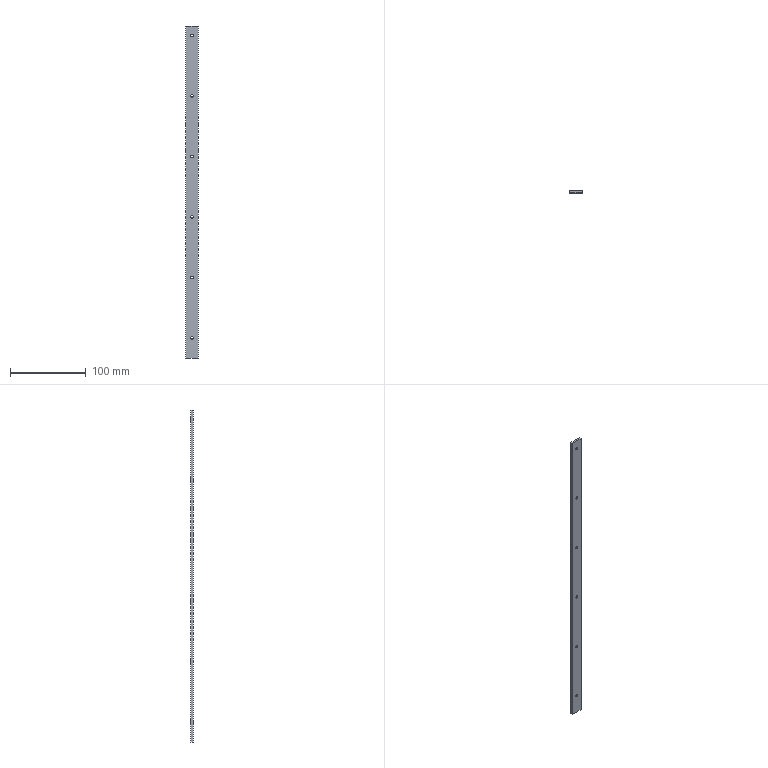Part | NX | features BREP 1 | 1 solid | 30 faces | box 16 x 3 x 439 mm | volume 20822 mm3 | cone 12 | cylinder 12 | plane 6 | commonest cylinder face diameters 3.4 x12
STEP:
#1=CARTESIAN_POINT('',(0.,1.5,203.85));
#2=VERTEX_POINT('',#1);
#3=CARTESIAN_POINT('',(0.,0.05,205.3));
#4=VERTEX_POINT('',#3);
#5=CARTESIAN_POINT('',(0.,1.5,203.85));
#6=DIRECTION('',(0.,0.7071,-0.7071));
#7=VECTOR('',#6,1000.);
#8=LINE('',#5,#7);
#9=EDGE_CURVE('',#2,#4,#8,.F.);
#10=ORIENTED_EDGE('',*,*,#9,.T.);
#11=CARTESIAN_POINT('',(0.,0.05,208.7));
#12=VERTEX_POINT('',#11);
#13=CARTESIAN_POINT('',(0.,0.05,207.));
#14=DIRECTION('',(0.,1.,0.));
#15=DIRECTION('',(0.,0.,1.));
#16=AXIS2_PLACEMENT_3D('',#13,#14,#15);
#17=CIRCLE('',#16,1.7);
#18=EDGE_CURVE('',#12,#4,#17,.T.);
#19=ORIENTED_EDGE('',*,*,#18,.F.);
#20=CARTESIAN_POINT('',(0.,1.5,210.15));
#21=VERTEX_POINT('',#20);
#22=CARTESIAN_POINT('',(0.,1.5,210.15));
#23=DIRECTION('',(0.,0.7071,0.7071));
#24=VECTOR('',#23,1000.);
#25=LINE('',#22,#24);
#26=EDGE_CURVE('',#21,#12,#25,.F.);
#27=ORIENTED_EDGE('',*,*,#26,.F.);
#28=CARTESIAN_POINT('',(0.,1.5,207.));
#29=DIRECTION('',(0.,1.,0.));
#30=DIRECTION('',(0.,0.,1.));
#31=AXIS2_PLACEMENT_3D('',#28,#29,#30);
#32=CIRCLE('',#31,3.15);
#33=EDGE_CURVE('',#21,#2,#32,.T.);
#34=ORIENTED_EDGE('',*,*,#33,.T.);
#35=EDGE_LOOP('',(#10,#19,#27,#34));
#36=FACE_BOUND('',#35,.T.);
#37=CARTESIAN_POINT('',(0.,1.5,207.));
#38=DIRECTION('',(0.,1.,0.));
#39=DIRECTION('',(0.,0.,1.));
#40=AXIS2_PLACEMENT_3D('',#37,#38,#39);
#41=CONICAL_SURFACE('',#40,3.15,0.7854);
#42=ADVANCED_FACE('',(#36),#41,.F.);
#43=CARTESIAN_POINT('',(0.,-1.5,205.3));
#44=VERTEX_POINT('',#43);
#45=CARTESIAN_POINT('',(0.,1.5,205.3));
#46=DIRECTION('',(0.,1.,0.));
#47=VECTOR('',#46,1000.);
#48=LINE('',#45,#47);
#49=EDGE_CURVE('',#4,#44,#48,.F.);
#50=ORIENTED_EDGE('',*,*,#49,.T.);
#51=CARTESIAN_POINT('',(0.,-1.5,208.7));
#52=VERTEX_POINT('',#51);
#53=CARTESIAN_POINT('',(0.,-1.5,207.));
#54=DIRECTION('',(0.,1.,0.));
#55=DIRECTION('',(0.,0.,1.));
#56=AXIS2_PLACEMENT_3D('',#53,#54,#55);
#57=CIRCLE('',#56,1.7);
#58=EDGE_CURVE('',#52,#44,#57,.T.);
#59=ORIENTED_EDGE('',*,*,#58,.F.);
#60=CARTESIAN_POINT('',(0.,1.5,208.7));
#61=DIRECTION('',(0.,1.,0.));
#62=VECTOR('',#61,1000.);
#63=LINE('',#60,#62);
#64=EDGE_CURVE('',#12,#52,#63,.F.);
#65=ORIENTED_EDGE('',*,*,#64,.F.);
#66=ORIENTED_EDGE('',*,*,#18,.T.);
#67=EDGE_LOOP('',(#50,#59,#65,#66));
#68=FACE_BOUND('',#67,.T.);
#69=CARTESIAN_POINT('',(0.,1.5,207.));
#70=DIRECTION('',(0.,1.,0.));
#71=DIRECTION('',(0.,0.,1.));
#72=AXIS2_PLACEMENT_3D('',#69,#70,#71);
#73=CYLINDRICAL_SURFACE('',#72,1.7);
#74=ADVANCED_FACE('',(#68),#73,.F.);
#75=CARTESIAN_POINT('',(0.,1.5,123.85));
#76=VERTEX_POINT('',#75);
#77=CARTESIAN_POINT('',(0.,0.05,125.3));
#78=VERTEX_POINT('',#77);
#79=CARTESIAN_POINT('',(0.,1.5,123.85));
#80=DIRECTION('',(0.,0.7071,-0.7071));
#81=VECTOR('',#80,1000.);
#82=LINE('',#79,#81);
#83=EDGE_CURVE('',#76,#78,#82,.F.);
#84=ORIENTED_EDGE('',*,*,#83,.T.);
#85=CARTESIAN_POINT('',(0.,0.05,128.7));
#86=VERTEX_POINT('',#85);
#87=CARTESIAN_POINT('',(0.,0.05,127.));
#88=DIRECTION('',(0.,1.,0.));
#89=DIRECTION('',(0.,0.,1.));
#90=AXIS2_PLACEMENT_3D('',#87,#88,#89);
#91=CIRCLE('',#90,1.7);
#92=EDGE_CURVE('',#86,#78,#91,.T.);
#93=ORIENTED_EDGE('',*,*,#92,.F.);
#94=CARTESIAN_POINT('',(0.,1.5,130.15));
#95=VERTEX_POINT('',#94);
#96=CARTESIAN_POINT('',(0.,1.5,130.15));
#97=DIRECTION('',(0.,0.7071,0.7071));
#98=VECTOR('',#97,1000.);
#99=LINE('',#96,#98);
#100=EDGE_CURVE('',#95,#86,#99,.F.);
#101=ORIENTED_EDGE('',*,*,#100,.F.);
#102=CARTESIAN_POINT('',(0.,1.5,127.));
#103=DIRECTION('',(0.,1.,0.));
#104=DIRECTION('',(0.,0.,1.));
#105=AXIS2_PLACEMENT_3D('',#102,#103,#104);
#106=CIRCLE('',#105,3.15);
#107=EDGE_CURVE('',#95,#76,#106,.T.);
#108=ORIENTED_EDGE('',*,*,#107,.T.);
#109=EDGE_LOOP('',(#84,#93,#101,#108));
#110=FACE_BOUND('',#109,.T.);
#111=CARTESIAN_POINT('',(0.,1.5,127.));
#112=DIRECTION('',(0.,1.,0.));
#113=DIRECTION('',(0.,0.,1.));
#114=AXIS2_PLACEMENT_3D('',#111,#112,#113);
#115=CONICAL_SURFACE('',#114,3.15,0.7854);
#116=ADVANCED_FACE('',(#110),#115,.F.);
#117=CARTESIAN_POINT('',(0.,-1.5,125.3));
#118=VERTEX_POINT('',#117);
#119=CARTESIAN_POINT('',(0.,1.5,125.3));
#120=DIRECTION('',(0.,1.,0.));
#121=VECTOR('',#120,1000.);
#122=LINE('',#119,#121);
#123=EDGE_CURVE('',#78,#118,#122,.F.);
#124=ORIENTED_EDGE('',*,*,#123,.T.);
#125=CARTESIAN_POINT('',(0.,-1.5,128.7));
#126=VERTEX_POINT('',#125);
#127=CARTESIAN_POINT('',(0.,-1.5,127.));
#128=DIRECTION('',(0.,1.,0.));
#129=DIRECTION('',(0.,0.,1.));
#130=AXIS2_PLACEMENT_3D('',#127,#128,#129);
#131=CIRCLE('',#130,1.7);
#132=EDGE_CURVE('',#126,#118,#131,.T.);
#133=ORIENTED_EDGE('',*,*,#132,.F.);
#134=CARTESIAN_POINT('',(0.,1.5,128.7));
#135=DIRECTION('',(0.,1.,0.));
#136=VECTOR('',#135,1000.);
#137=LINE('',#134,#136);
#138=EDGE_CURVE('',#86,#126,#137,.F.);
#139=ORIENTED_EDGE('',*,*,#138,.F.);
#140=ORIENTED_EDGE('',*,*,#92,.T.);
#141=EDGE_LOOP('',(#124,#133,#139,#140));
#142=FACE_BOUND('',#141,.T.);
#143=CARTESIAN_POINT('',(0.,1.5,127.));
#144=DIRECTION('',(0.,1.,0.));
#145=DIRECTION('',(0.,0.,1.));
#146=AXIS2_PLACEMENT_3D('',#143,#144,#145);
#147=CYLINDRICAL_SURFACE('',#146,1.7);
#148=ADVANCED_FACE('',(#142),#147,.F.);
#149=CARTESIAN_POINT('',(0.,1.5,43.85));
#150=VERTEX_POINT('',#149);
#151=CARTESIAN_POINT('',(0.,0.05,45.3));
#152=VERTEX_POINT('',#151);
#153=CARTESIAN_POINT('',(0.,1.5,43.85));
#154=DIRECTION('',(0.,0.7071,-0.7071));
#155=VECTOR('',#154,1000.);
#156=LINE('',#153,#155);
#157=EDGE_CURVE('',#150,#152,#156,.F.);
#158=ORIENTED_EDGE('',*,*,#157,.T.);
#159=CARTESIAN_POINT('',(0.,0.05,48.7));
#160=VERTEX_POINT('',#159);
#161=CARTESIAN_POINT('',(0.,0.05,47.));
#162=DIRECTION('',(0.,1.,0.));
#163=DIRECTION('',(0.,0.,1.));
#164=AXIS2_PLACEMENT_3D('',#161,#162,#163);
#165=CIRCLE('',#164,1.7);
#166=EDGE_CURVE('',#160,#152,#165,.T.);
#167=ORIENTED_EDGE('',*,*,#166,.F.);
#168=CARTESIAN_POINT('',(0.,1.5,50.15));
#169=VERTEX_POINT('',#168);
#170=CARTESIAN_POINT('',(0.,1.5,50.15));
#171=DIRECTION('',(0.,0.7071,0.7071));
#172=VECTOR('',#171,1000.);
#173=LINE('',#170,#172);
#174=EDGE_CURVE('',#169,#160,#173,.F.);
#175=ORIENTED_EDGE('',*,*,#174,.F.);
#176=CARTESIAN_POINT('',(0.,1.5,47.));
#177=DIRECTION('',(0.,1.,0.));
#178=DIRECTION('',(0.,0.,1.));
#179=AXIS2_PLACEMENT_3D('',#176,#177,#178);
#180=CIRCLE('',#179,3.15);
#181=EDGE_CURVE('',#169,#150,#180,.T.);
#182=ORIENTED_EDGE('',*,*,#181,.T.);
#183=EDGE_LOOP('',(#158,#167,#175,#182));
#184=FACE_BOUND('',#183,.T.);
#185=CARTESIAN_POINT('',(0.,1.5,47.));
#186=DIRECTION('',(0.,1.,0.));
#187=DIRECTION('',(0.,0.,1.));
#188=AXIS2_PLACEMENT_3D('',#185,#186,#187);
#189=CONICAL_SURFACE('',#188,3.15,0.7854);
#190=ADVANCED_FACE('',(#184),#189,.F.);
#191=CARTESIAN_POINT('',(0.,-1.5,45.3));
#192=VERTEX_POINT('',#191);
#193=CARTESIAN_POINT('',(0.,1.5,45.3));
#194=DIRECTION('',(0.,1.,0.));
#195=VECTOR('',#194,1000.);
#196=LINE('',#193,#195);
#197=EDGE_CURVE('',#152,#192,#196,.F.);
#198=ORIENTED_EDGE('',*,*,#197,.T.);
#199=CARTESIAN_POINT('',(0.,-1.5,48.7));
#200=VERTEX_POINT('',#199);
#201=CARTESIAN_POINT('',(0.,-1.5,47.));
#202=DIRECTION('',(0.,1.,0.));
#203=DIRECTION('',(0.,0.,1.));
#204=AXIS2_PLACEMENT_3D('',#201,#202,#203);
#205=CIRCLE('',#204,1.7);
#206=EDGE_CURVE('',#200,#192,#205,.T.);
#207=ORIENTED_EDGE('',*,*,#206,.F.);
#208=CARTESIAN_POINT('',(0.,1.5,48.7));
#209=DIRECTION('',(0.,1.,0.));
#210=VECTOR('',#209,1000.);
#211=LINE('',#208,#210);
#212=EDGE_CURVE('',#160,#200,#211,.F.);
#213=ORIENTED_EDGE('',*,*,#212,.F.);
#214=ORIENTED_EDGE('',*,*,#166,.T.);
#215=EDGE_LOOP('',(#198,#207,#213,#214));
#216=FACE_BOUND('',#215,.T.);
#217=CARTESIAN_POINT('',(0.,1.5,47.));
#218=DIRECTION('',(0.,1.,0.));
#219=DIRECTION('',(0.,0.,1.));
#220=AXIS2_PLACEMENT_3D('',#217,#218,#219);
#221=CYLINDRICAL_SURFACE('',#220,1.7);
#222=ADVANCED_FACE('',(#216),#221,.F.);
#223=CARTESIAN_POINT('',(0.,1.5,-36.15));
#224=VERTEX_POINT('',#223);
#225=CARTESIAN_POINT('',(0.,0.05,-34.7));
#226=VERTEX_POINT('',#225);
#227=CARTESIAN_POINT('',(0.,1.5,-36.15));
#228=DIRECTION('',(0.,0.7071,-0.7071));
#229=VECTOR('',#228,1000.);
#230=LINE('',#227,#229);
#231=EDGE_CURVE('',#224,#226,#230,.F.);
#232=ORIENTED_EDGE('',*,*,#231,.T.);
#233=CARTESIAN_POINT('',(0.,0.05,-31.3));
#234=VERTEX_POINT('',#233);
#235=CARTESIAN_POINT('',(0.,0.05,-33.));
#236=DIRECTION('',(0.,1.,0.));
#237=DIRECTION('',(0.,0.,1.));
#238=AXIS2_PLACEMENT_3D('',#235,#236,#237);
#239=CIRCLE('',#238,1.7);
#240=EDGE_CURVE('',#234,#226,#239,.T.);
#241=ORIENTED_EDGE('',*,*,#240,.F.);
#242=CARTESIAN_POINT('',(0.,1.5,-29.85));
#243=VERTEX_POINT('',#242);
#244=CARTESIAN_POINT('',(0.,1.5,-29.85));
#245=DIRECTION('',(0.,0.7071,0.7071));
#246=VECTOR('',#245,1000.);
#247=LINE('',#244,#246);
#248=EDGE_CURVE('',#243,#234,#247,.F.);
#249=ORIENTED_EDGE('',*,*,#248,.F.);
#250=CARTESIAN_POINT('',(0.,1.5,-33.));
#251=DIRECTION('',(0.,1.,0.));
#252=DIRECTION('',(0.,0.,1.));
#253=AXIS2_PLACEMENT_3D('',#250,#251,#252);
#254=CIRCLE('',#253,3.15);
#255=EDGE_CURVE('',#243,#224,#254,.T.);
#256=ORIENTED_EDGE('',*,*,#255,.T.);
#257=EDGE_LOOP('',(#232,#241,#249,#256));
#258=FACE_BOUND('',#257,.T.);
#259=CARTESIAN_POINT('',(0.,1.5,-33.));
#260=DIRECTION('',(0.,1.,0.));
#261=DIRECTION('',(0.,0.,1.));
#262=AXIS2_PLACEMENT_3D('',#259,#260,#261);
#263=CONICAL_SURFACE('',#262,3.15,0.7854);
#264=ADVANCED_FACE('',(#258),#263,.F.);
#265=CARTESIAN_POINT('',(0.,-1.5,-34.7));
#266=VERTEX_POINT('',#265);
#267=CARTESIAN_POINT('',(0.,1.5,-34.7));
#268=DIRECTION('',(0.,1.,0.));
#269=VECTOR('',#268,1000.);
#270=LINE('',#267,#269);
#271=EDGE_CURVE('',#226,#266,#270,.F.);
#272=ORIENTED_EDGE('',*,*,#271,.T.);
#273=CARTESIAN_POINT('',(0.,-1.5,-31.3));
#274=VERTEX_POINT('',#273);
#275=CARTESIAN_POINT('',(0.,-1.5,-33.));
#276=DIRECTION('',(0.,1.,0.));
#277=DIRECTION('',(0.,0.,1.));
#278=AXIS2_PLACEMENT_3D('',#275,#276,#277);
#279=CIRCLE('',#278,1.7);
#280=EDGE_CURVE('',#274,#266,#279,.T.);
#281=ORIENTED_EDGE('',*,*,#280,.F.);
#282=CARTESIAN_POINT('',(0.,1.5,-31.3));
#283=DIRECTION('',(0.,1.,0.));
#284=VECTOR('',#283,1000.);
#285=LINE('',#282,#284);
#286=EDGE_CURVE('',#234,#274,#285,.F.);
#287=ORIENTED_EDGE('',*,*,#286,.F.);
#288=ORIENTED_EDGE('',*,*,#240,.T.);
#289=EDGE_LOOP('',(#272,#281,#287,#288));
#290=FACE_BOUND('',#289,.T.);
#291=CARTESIAN_POINT('',(0.,1.5,-33.));
#292=DIRECTION('',(0.,1.,0.));
#293=DIRECTION('',(0.,0.,1.));
#294=AXIS2_PLACEMENT_3D('',#291,#292,#293);
#295=CYLINDRICAL_SURFACE('',#294,1.7);
#296=ADVANCED_FACE('',(#290),#295,.F.);
#297=CARTESIAN_POINT('',(0.,1.5,-116.15));
#298=VERTEX_POINT('',#297);
#299=CARTESIAN_POINT('',(0.,0.05,-114.7));
#300=VERTEX_POINT('',#299);
#301=CARTESIAN_POINT('',(0.,1.5,-116.15));
#302=DIRECTION('',(0.,0.7071,-0.7071));
#303=VECTOR('',#302,1000.);
#304=LINE('',#301,#303);
#305=EDGE_CURVE('',#298,#300,#304,.F.);
#306=ORIENTED_EDGE('',*,*,#305,.T.);
#307=CARTESIAN_POINT('',(0.,0.05,-111.3));
#308=VERTEX_POINT('',#307);
#309=CARTESIAN_POINT('',(0.,0.05,-113.));
#310=DIRECTION('',(0.,1.,0.));
#311=DIRECTION('',(0.,0.,1.));
#312=AXIS2_PLACEMENT_3D('',#309,#310,#311);
#313=CIRCLE('',#312,1.7);
#314=EDGE_CURVE('',#308,#300,#313,.T.);
#315=ORIENTED_EDGE('',*,*,#314,.F.);
#316=CARTESIAN_POINT('',(0.,1.5,-109.85));
#317=VERTEX_POINT('',#316);
#318=CARTESIAN_POINT('',(0.,1.5,-109.85));
#319=DIRECTION('',(0.,0.7071,0.7071));
#320=VECTOR('',#319,1000.);
#321=LINE('',#318,#320);
#322=EDGE_CURVE('',#317,#308,#321,.F.);
#323=ORIENTED_EDGE('',*,*,#322,.F.);
#324=CARTESIAN_POINT('',(0.,1.5,-113.));
#325=DIRECTION('',(0.,1.,0.));
#326=DIRECTION('',(0.,0.,1.));
#327=AXIS2_PLACEMENT_3D('',#324,#325,#326);
#328=CIRCLE('',#327,3.15);
#329=EDGE_CURVE('',#317,#298,#328,.T.);
#330=ORIENTED_EDGE('',*,*,#329,.T.);
#331=EDGE_LOOP('',(#306,#315,#323,#330));
#332=FACE_BOUND('',#331,.T.);
#333=CARTESIAN_POINT('',(0.,1.5,-113.));
#334=DIRECTION('',(0.,1.,0.));
#335=DIRECTION('',(0.,0.,1.));
#336=AXIS2_PLACEMENT_3D('',#333,#334,#335);
#337=CONICAL_SURFACE('',#336,3.15,0.7854);
#338=ADVANCED_FACE('',(#332),#337,.F.);
#339=CARTESIAN_POINT('',(0.,-1.5,-114.7));
#340=VERTEX_POINT('',#339);
#341=CARTESIAN_POINT('',(0.,1.5,-114.7));
#342=DIRECTION('',(0.,1.,0.));
#343=VECTOR('',#342,1000.);
#344=LINE('',#341,#343);
#345=EDGE_CURVE('',#300,#340,#344,.F.);
#346=ORIENTED_EDGE('',*,*,#345,.T.);
#347=CARTESIAN_POINT('',(0.,-1.5,-111.3));
#348=VERTEX_POINT('',#347);
#349=CARTESIAN_POINT('',(0.,-1.5,-113.));
#350=DIRECTION('',(0.,1.,0.));
#351=DIRECTION('',(0.,0.,1.));
#352=AXIS2_PLACEMENT_3D('',#349,#350,#351);
#353=CIRCLE('',#352,1.7);
#354=EDGE_CURVE('',#348,#340,#353,.T.);
#355=ORIENTED_EDGE('',*,*,#354,.F.);
#356=CARTESIAN_POINT('',(0.,1.5,-111.3));
#357=DIRECTION('',(0.,1.,0.));
#358=VECTOR('',#357,1000.);
#359=LINE('',#356,#358);
#360=EDGE_CURVE('',#308,#348,#359,.F.);
#361=ORIENTED_EDGE('',*,*,#360,.F.);
#362=ORIENTED_EDGE('',*,*,#314,.T.);
#363=EDGE_LOOP('',(#346,#355,#361,#362));
#364=FACE_BOUND('',#363,.T.);
#365=CARTESIAN_POINT('',(0.,1.5,-113.));
#366=DIRECTION('',(0.,1.,0.));
#367=DIRECTION('',(0.,0.,1.));
#368=AXIS2_PLACEMENT_3D('',#365,#366,#367);
#369=CYLINDRICAL_SURFACE('',#368,1.7);
#370=ADVANCED_FACE('',(#364),#369,.F.);
#371=CARTESIAN_POINT('',(0.,1.5,-196.15));
#372=VERTEX_POINT('',#371);
#373=CARTESIAN_POINT('',(0.,0.05,-194.7));
#374=VERTEX_POINT('',#373);
#375=CARTESIAN_POINT('',(0.,1.5,-196.15));
#376=DIRECTION('',(0.,0.7071,-0.7071));
#377=VECTOR('',#376,1000.);
#378=LINE('',#375,#377);
#379=EDGE_CURVE('',#372,#374,#378,.F.);
#380=ORIENTED_EDGE('',*,*,#379,.T.);
#381=CARTESIAN_POINT('',(0.,0.05,-191.3));
#382=VERTEX_POINT('',#381);
#383=CARTESIAN_POINT('',(0.,0.05,-193.));
#384=DIRECTION('',(0.,1.,0.));
#385=DIRECTION('',(0.,0.,1.));
#386=AXIS2_PLACEMENT_3D('',#383,#384,#385);
#387=CIRCLE('',#386,1.7);
#388=EDGE_CURVE('',#382,#374,#387,.T.);
#389=ORIENTED_EDGE('',*,*,#388,.F.);
#390=CARTESIAN_POINT('',(0.,1.5,-189.85));
#391=VERTEX_POINT('',#390);
#392=CARTESIAN_POINT('',(0.,1.5,-189.85));
#393=DIRECTION('',(0.,0.7071,0.7071));
#394=VECTOR('',#393,1000.);
#395=LINE('',#392,#394);
#396=EDGE_CURVE('',#391,#382,#395,.F.);
#397=ORIENTED_EDGE('',*,*,#396,.F.);
#398=CARTESIAN_POINT('',(0.,1.5,-193.));
#399=DIRECTION('',(0.,1.,0.));
#400=DIRECTION('',(0.,0.,1.));
#401=AXIS2_PLACEMENT_3D('',#398,#399,#400);
#402=CIRCLE('',#401,3.15);
#403=EDGE_CURVE('',#391,#372,#402,.T.);
#404=ORIENTED_EDGE('',*,*,#403,.T.);
#405=EDGE_LOOP('',(#380,#389,#397,#404));
#406=FACE_BOUND('',#405,.T.);
#407=CARTESIAN_POINT('',(0.,1.5,-193.));
#408=DIRECTION('',(0.,1.,0.));
#409=DIRECTION('',(0.,0.,1.));
#410=AXIS2_PLACEMENT_3D('',#407,#408,#409);
#411=CONICAL_SURFACE('',#410,3.15,0.7854);
#412=ADVANCED_FACE('',(#406),#411,.F.);
#413=CARTESIAN_POINT('',(0.,-1.5,-194.7));
#414=VERTEX_POINT('',#413);
#415=CARTESIAN_POINT('',(0.,1.5,-194.7));
#416=DIRECTION('',(0.,1.,0.));
#417=VECTOR('',#416,1000.);
#418=LINE('',#415,#417);
#419=EDGE_CURVE('',#374,#414,#418,.F.);
#420=ORIENTED_EDGE('',*,*,#419,.T.);
#421=CARTESIAN_POINT('',(0.,-1.5,-191.3));
#422=VERTEX_POINT('',#421);
#423=CARTESIAN_POINT('',(0.,-1.5,-193.));
#424=DIRECTION('',(0.,1.,0.));
#425=DIRECTION('',(0.,0.,1.));
#426=AXIS2_PLACEMENT_3D('',#423,#424,#425);
#427=CIRCLE('',#426,1.7);
#428=EDGE_CURVE('',#422,#414,#427,.T.);
#429=ORIENTED_EDGE('',*,*,#428,.F.);
#430=CARTESIAN_POINT('',(0.,1.5,-191.3));
#431=DIRECTION('',(0.,1.,0.));
#432=VECTOR('',#431,1000.);
#433=LINE('',#430,#432);
#434=EDGE_CURVE('',#382,#422,#433,.F.);
#435=ORIENTED_EDGE('',*,*,#434,.F.);
#436=ORIENTED_EDGE('',*,*,#388,.T.);
#437=EDGE_LOOP('',(#420,#429,#435,#436));
#438=FACE_BOUND('',#437,.T.);
#439=CARTESIAN_POINT('',(0.,1.5,-193.));
#440=DIRECTION('',(0.,1.,0.));
#441=DIRECTION('',(0.,0.,1.));
#442=AXIS2_PLACEMENT_3D('',#439,#440,#441);
#443=CYLINDRICAL_SURFACE('',#442,1.7);
#444=ADVANCED_FACE('',(#438),#443,.F.);
#445=CARTESIAN_POINT('',(8.,-1.5,-219.5));
#446=VERTEX_POINT('',#445);
#447=CARTESIAN_POINT('',(8.,1.5,-219.5));
#448=VERTEX_POINT('',#447);
#449=CARTESIAN_POINT('',(8.,-1.5,-219.5));
#450=DIRECTION('',(0.,1.,0.));
#451=VECTOR('',#450,1000.);
#452=LINE('',#449,#451);
#453=EDGE_CURVE('',#446,#448,#452,.T.);
#454=ORIENTED_EDGE('',*,*,#453,.F.);
#455=CARTESIAN_POINT('',(-8.,-1.5,-219.5));
#456=VERTEX_POINT('',#455);
#457=CARTESIAN_POINT('',(-8.,-1.5,-219.5));
#458=DIRECTION('',(1.,0.,0.));
#459=VECTOR('',#458,1000.);
#460=LINE('',#457,#459);
#461=EDGE_CURVE('',#456,#446,#460,.T.);
#462=ORIENTED_EDGE('',*,*,#461,.F.);
#463=CARTESIAN_POINT('',(-8.,1.5,-219.5));
#464=VERTEX_POINT('',#463);
#465=CARTESIAN_POINT('',(-8.,-1.5,-219.5));
#466=DIRECTION('',(0.,-1.,0.));
#467=VECTOR('',#466,1000.);
#468=LINE('',#465,#467);
#469=EDGE_CURVE('',#464,#456,#468,.T.);
#470=ORIENTED_EDGE('',*,*,#469,.F.);
#471=CARTESIAN_POINT('',(-8.,1.5,-219.5));
#472=DIRECTION('',(-1.,0.,0.));
#473=VECTOR('',#472,1000.);
#474=LINE('',#471,#473);
#475=EDGE_CURVE('',#448,#464,#474,.T.);
#476=ORIENTED_EDGE('',*,*,#475,.F.);
#477=EDGE_LOOP('',(#454,#462,#470,#476));
#478=FACE_BOUND('',#477,.T.);
#479=CARTESIAN_POINT('',(0.,0.,-219.5));
#480=DIRECTION('',(0.,0.,-1.));
#481=DIRECTION('',(-1.,0.,0.));
#482=AXIS2_PLACEMENT_3D('',#479,#480,#481);
#483=PLANE('',#482);
#484=ADVANCED_FACE('',(#478),#483,.T.);
#485=CARTESIAN_POINT('',(8.,-1.5,219.5));
#486=VERTEX_POINT('',#485);
#487=CARTESIAN_POINT('',(8.,1.5,219.5));
#488=VERTEX_POINT('',#487);
#489=CARTESIAN_POINT('',(8.,-1.5,219.5));
#490=DIRECTION('',(0.,1.,0.));
#491=VECTOR('',#490,1000.);
#492=LINE('',#489,#491);
#493=EDGE_CURVE('',#486,#488,#492,.T.);
#494=ORIENTED_EDGE('',*,*,#493,.T.);
#495=CARTESIAN_POINT('',(-8.,1.5,219.5));
#496=VERTEX_POINT('',#495);
#497=CARTESIAN_POINT('',(-8.,1.5,219.5));
#498=DIRECTION('',(-1.,0.,0.));
#499=VECTOR('',#498,1000.);
#500=LINE('',#497,#499);
#501=EDGE_CURVE('',#488,#496,#500,.T.);
#502=ORIENTED_EDGE('',*,*,#501,.T.);
#503=CARTESIAN_POINT('',(-8.,-1.5,219.5));
#504=VERTEX_POINT('',#503);
#505=CARTESIAN_POINT('',(-8.,-1.5,219.5));
#506=DIRECTION('',(0.,-1.,0.));
#507=VECTOR('',#506,1000.);
#508=LINE('',#505,#507);
#509=EDGE_CURVE('',#496,#504,#508,.T.);
#510=ORIENTED_EDGE('',*,*,#509,.T.);
#511=CARTESIAN_POINT('',(-8.,-1.5,219.5));
#512=DIRECTION('',(1.,0.,0.));
#513=VECTOR('',#512,1000.);
#514=LINE('',#511,#513);
#515=EDGE_CURVE('',#504,#486,#514,.T.);
#516=ORIENTED_EDGE('',*,*,#515,.T.);
#517=EDGE_LOOP('',(#494,#502,#510,#516));
#518=FACE_BOUND('',#517,.T.);
#519=CARTESIAN_POINT('',(0.,0.,219.5));
#520=DIRECTION('',(0.,0.,-1.));
#521=DIRECTION('',(-1.,0.,0.));
#522=AXIS2_PLACEMENT_3D('',#519,#520,#521);
#523=PLANE('',#522);
#524=ADVANCED_FACE('',(#518),#523,.F.);
#525=ORIENTED_EDGE('',*,*,#461,.T.);
#526=CARTESIAN_POINT('',(8.,-1.5,219.5));
#527=DIRECTION('',(0.,0.,-1.));
#528=VECTOR('',#527,1000.);
#529=LINE('',#526,#528);
#530=EDGE_CURVE('',#486,#446,#529,.T.);
#531=ORIENTED_EDGE('',*,*,#530,.F.);
#532=ORIENTED_EDGE('',*,*,#515,.F.);
#533=CARTESIAN_POINT('',(-8.,-1.5,219.5));
#534=DIRECTION('',(0.,0.,-1.));
#535=VECTOR('',#534,1000.);
#536=LINE('',#533,#535);
#537=EDGE_CURVE('',#504,#456,#536,.T.);
#538=ORIENTED_EDGE('',*,*,#537,.T.);
#539=EDGE_LOOP('',(#525,#531,#532,#538));
#540=FACE_BOUND('',#539,.T.);
#541=ORIENTED_EDGE('',*,*,#428,.T.);
#542=CARTESIAN_POINT('',(0.,-1.5,-193.));
#543=DIRECTION('',(0.,1.,0.));
#544=DIRECTION('',(0.,0.,1.));
#545=AXIS2_PLACEMENT_3D('',#542,#543,#544);
#546=CIRCLE('',#545,1.7);
#547=EDGE_CURVE('',#414,#422,#546,.T.);
#548=ORIENTED_EDGE('',*,*,#547,.T.);
#549=EDGE_LOOP('',(#541,#548));
#550=FACE_BOUND('',#549,.T.);
#551=ORIENTED_EDGE('',*,*,#354,.T.);
#552=CARTESIAN_POINT('',(0.,-1.5,-113.));
#553=DIRECTION('',(0.,1.,0.));
#554=DIRECTION('',(0.,0.,1.));
#555=AXIS2_PLACEMENT_3D('',#552,#553,#554);
#556=CIRCLE('',#555,1.7);
#557=EDGE_CURVE('',#340,#348,#556,.T.);
#558=ORIENTED_EDGE('',*,*,#557,.T.);
#559=EDGE_LOOP('',(#551,#558));
#560=FACE_BOUND('',#559,.T.);
#561=ORIENTED_EDGE('',*,*,#280,.T.);
#562=CARTESIAN_POINT('',(0.,-1.5,-33.));
#563=DIRECTION('',(0.,1.,0.));
#564=DIRECTION('',(0.,0.,1.));
#565=AXIS2_PLACEMENT_3D('',#562,#563,#564);
#566=CIRCLE('',#565,1.7);
#567=EDGE_CURVE('',#266,#274,#566,.T.);
#568=ORIENTED_EDGE('',*,*,#567,.T.);
#569=EDGE_LOOP('',(#561,#568));
#570=FACE_BOUND('',#569,.T.);
#571=ORIENTED_EDGE('',*,*,#206,.T.);
#572=CARTESIAN_POINT('',(0.,-1.5,47.));
#573=DIRECTION('',(0.,1.,0.));
#574=DIRECTION('',(0.,0.,1.));
#575=AXIS2_PLACEMENT_3D('',#572,#573,#574);
#576=CIRCLE('',#575,1.7);
#577=EDGE_CURVE('',#192,#200,#576,.T.);
#578=ORIENTED_EDGE('',*,*,#577,.T.);
#579=EDGE_LOOP('',(#571,#578));
#580=FACE_BOUND('',#579,.T.);
#581=ORIENTED_EDGE('',*,*,#132,.T.);
#582=CARTESIAN_POINT('',(0.,-1.5,127.));
#583=DIRECTION('',(0.,1.,0.));
#584=DIRECTION('',(0.,0.,1.));
#585=AXIS2_PLACEMENT_3D('',#582,#583,#584);
#586=CIRCLE('',#585,1.7);
#587=EDGE_CURVE('',#118,#126,#586,.T.);
#588=ORIENTED_EDGE('',*,*,#587,.T.);
#589=EDGE_LOOP('',(#581,#588));
#590=FACE_BOUND('',#589,.T.);
#591=ORIENTED_EDGE('',*,*,#58,.T.);
#592=CARTESIAN_POINT('',(0.,-1.5,207.));
#593=DIRECTION('',(0.,1.,0.));
#594=DIRECTION('',(0.,0.,1.));
#595=AXIS2_PLACEMENT_3D('',#592,#593,#594);
#596=CIRCLE('',#595,1.7);
#597=EDGE_CURVE('',#44,#52,#596,.T.);
#598=ORIENTED_EDGE('',*,*,#597,.T.);
#599=EDGE_LOOP('',(#591,#598));
#600=FACE_BOUND('',#599,.T.);
#601=CARTESIAN_POINT('',(-8.,-1.5,219.5));
#602=DIRECTION('',(0.,1.,0.));
#603=DIRECTION('',(0.,0.,1.));
#604=AXIS2_PLACEMENT_3D('',#601,#602,#603);
#605=PLANE('',#604);
#606=ADVANCED_FACE('',(#540,#550,#560,#570,#580,#590,#600),#605,.F.);
#607=ORIENTED_EDGE('',*,*,#469,.T.);
#608=ORIENTED_EDGE('',*,*,#537,.F.);
#609=ORIENTED_EDGE('',*,*,#509,.F.);
#610=CARTESIAN_POINT('',(-8.,1.5,219.5));
#611=DIRECTION('',(0.,0.,-1.));
#612=VECTOR('',#611,1000.);
#613=LINE('',#610,#612);
#614=EDGE_CURVE('',#496,#464,#613,.T.);
#615=ORIENTED_EDGE('',*,*,#614,.T.);
#616=EDGE_LOOP('',(#607,#608,#609,#615));
#617=FACE_BOUND('',#616,.T.);
#618=CARTESIAN_POINT('',(-8.,-1.5,219.5));
#619=DIRECTION('',(1.,0.,0.));
#620=DIRECTION('',(0.,0.,-1.));
#621=AXIS2_PLACEMENT_3D('',#618,#619,#620);
#622=PLANE('',#621);
#623=ADVANCED_FACE('',(#617),#622,.F.);
#624=ORIENTED_EDGE('',*,*,#475,.T.);
#625=ORIENTED_EDGE('',*,*,#614,.F.);
#626=ORIENTED_EDGE('',*,*,#501,.F.);
#627=CARTESIAN_POINT('',(8.,1.5,219.5));
#628=DIRECTION('',(0.,0.,-1.));
#629=VECTOR('',#628,1000.);
#630=LINE('',#627,#629);
#631=EDGE_CURVE('',#488,#448,#630,.T.);
#632=ORIENTED_EDGE('',*,*,#631,.T.);
#633=EDGE_LOOP('',(#624,#625,#626,#632));
#634=FACE_BOUND('',#633,.T.);
#635=ORIENTED_EDGE('',*,*,#403,.F.);
#636=CARTESIAN_POINT('',(0.,1.5,-193.));
#637=DIRECTION('',(0.,1.,0.));
#638=DIRECTION('',(0.,0.,1.));
#639=AXIS2_PLACEMENT_3D('',#636,#637,#638);
#640=CIRCLE('',#639,3.15);
#641=EDGE_CURVE('',#372,#391,#640,.T.);
#642=ORIENTED_EDGE('',*,*,#641,.F.);
#643=EDGE_LOOP('',(#635,#642));
#644=FACE_BOUND('',#643,.T.);
#645=ORIENTED_EDGE('',*,*,#329,.F.);
#646=CARTESIAN_POINT('',(0.,1.5,-113.));
#647=DIRECTION('',(0.,1.,0.));
#648=DIRECTION('',(0.,0.,1.));
#649=AXIS2_PLACEMENT_3D('',#646,#647,#648);
#650=CIRCLE('',#649,3.15);
#651=EDGE_CURVE('',#298,#317,#650,.T.);
#652=ORIENTED_EDGE('',*,*,#651,.F.);
#653=EDGE_LOOP('',(#645,#652));
#654=FACE_BOUND('',#653,.T.);
#655=ORIENTED_EDGE('',*,*,#255,.F.);
#656=CARTESIAN_POINT('',(0.,1.5,-33.));
#657=DIRECTION('',(0.,1.,0.));
#658=DIRECTION('',(0.,0.,1.));
#659=AXIS2_PLACEMENT_3D('',#656,#657,#658);
#660=CIRCLE('',#659,3.15);
#661=EDGE_CURVE('',#224,#243,#660,.T.);
#662=ORIENTED_EDGE('',*,*,#661,.F.);
#663=EDGE_LOOP('',(#655,#662));
#664=FACE_BOUND('',#663,.T.);
#665=ORIENTED_EDGE('',*,*,#181,.F.);
#666=CARTESIAN_POINT('',(0.,1.5,47.));
#667=DIRECTION('',(0.,1.,0.));
#668=DIRECTION('',(0.,0.,1.));
#669=AXIS2_PLACEMENT_3D('',#666,#667,#668);
#670=CIRCLE('',#669,3.15);
#671=EDGE_CURVE('',#150,#169,#670,.T.);
#672=ORIENTED_EDGE('',*,*,#671,.F.);
#673=EDGE_LOOP('',(#665,#672));
#674=FACE_BOUND('',#673,.T.);
#675=ORIENTED_EDGE('',*,*,#107,.F.);
#676=CARTESIAN_POINT('',(0.,1.5,127.));
#677=DIRECTION('',(0.,1.,0.));
#678=DIRECTION('',(0.,0.,1.));
#679=AXIS2_PLACEMENT_3D('',#676,#677,#678);
#680=CIRCLE('',#679,3.15);
#681=EDGE_CURVE('',#76,#95,#680,.T.);
#682=ORIENTED_EDGE('',*,*,#681,.F.);
#683=EDGE_LOOP('',(#675,#682));
#684=FACE_BOUND('',#683,.T.);
#685=ORIENTED_EDGE('',*,*,#33,.F.);
#686=CARTESIAN_POINT('',(0.,1.5,207.));
#687=DIRECTION('',(0.,1.,0.));
#688=DIRECTION('',(0.,0.,1.));
#689=AXIS2_PLACEMENT_3D('',#686,#687,#688);
#690=CIRCLE('',#689,3.15);
#691=EDGE_CURVE('',#2,#21,#690,.T.);
#692=ORIENTED_EDGE('',*,*,#691,.F.);
#693=EDGE_LOOP('',(#685,#692));
#694=FACE_BOUND('',#693,.T.);
#695=CARTESIAN_POINT('',(-8.,1.5,219.5));
#696=DIRECTION('',(0.,-1.,0.));
#697=DIRECTION('',(0.,0.,-1.));
#698=AXIS2_PLACEMENT_3D('',#695,#696,#697);
#699=PLANE('',#698);
#700=ADVANCED_FACE('',(#634,#644,#654,#664,#674,#684,#694),#699,.F.);
#701=ORIENTED_EDGE('',*,*,#453,.T.);
#702=ORIENTED_EDGE('',*,*,#631,.F.);
#703=ORIENTED_EDGE('',*,*,#493,.F.);
#704=ORIENTED_EDGE('',*,*,#530,.T.);
#705=EDGE_LOOP('',(#701,#702,#703,#704));
#706=FACE_BOUND('',#705,.T.);
#707=CARTESIAN_POINT('',(8.,-1.5,219.5));
#708=DIRECTION('',(-1.,0.,0.));
#709=DIRECTION('',(0.,0.,1.));
#710=AXIS2_PLACEMENT_3D('',#707,#708,#709);
#711=PLANE('',#710);
#712=ADVANCED_FACE('',(#706),#711,.F.);
#713=ORIENTED_EDGE('',*,*,#547,.F.);
#714=ORIENTED_EDGE('',*,*,#419,.F.);
#715=CARTESIAN_POINT('',(0.,0.05,-193.));
#716=DIRECTION('',(0.,1.,0.));
#717=DIRECTION('',(0.,0.,1.));
#718=AXIS2_PLACEMENT_3D('',#715,#716,#717);
#719=CIRCLE('',#718,1.7);
#720=EDGE_CURVE('',#374,#382,#719,.T.);
#721=ORIENTED_EDGE('',*,*,#720,.T.);
#722=ORIENTED_EDGE('',*,*,#434,.T.);
#723=EDGE_LOOP('',(#713,#714,#721,#722));
#724=FACE_BOUND('',#723,.T.);
#725=CARTESIAN_POINT('',(0.,1.5,-193.));
#726=DIRECTION('',(0.,1.,0.));
#727=DIRECTION('',(0.,0.,1.));
#728=AXIS2_PLACEMENT_3D('',#725,#726,#727);
#729=CYLINDRICAL_SURFACE('',#728,1.7);
#730=ADVANCED_FACE('',(#724),#729,.F.);
#731=ORIENTED_EDGE('',*,*,#720,.F.);
#732=ORIENTED_EDGE('',*,*,#379,.F.);
#733=ORIENTED_EDGE('',*,*,#641,.T.);
#734=ORIENTED_EDGE('',*,*,#396,.T.);
#735=EDGE_LOOP('',(#731,#732,#733,#734));
#736=FACE_BOUND('',#735,.T.);
#737=CARTESIAN_POINT('',(0.,1.5,-193.));
#738=DIRECTION('',(0.,1.,0.));
#739=DIRECTION('',(0.,0.,1.));
#740=AXIS2_PLACEMENT_3D('',#737,#738,#739);
#741=CONICAL_SURFACE('',#740,3.15,0.7854);
#742=ADVANCED_FACE('',(#736),#741,.F.);
#743=ORIENTED_EDGE('',*,*,#557,.F.);
#744=ORIENTED_EDGE('',*,*,#345,.F.);
#745=CARTESIAN_POINT('',(0.,0.05,-113.));
#746=DIRECTION('',(0.,1.,0.));
#747=DIRECTION('',(0.,0.,1.));
#748=AXIS2_PLACEMENT_3D('',#745,#746,#747);
#749=CIRCLE('',#748,1.7);
#750=EDGE_CURVE('',#300,#308,#749,.T.);
#751=ORIENTED_EDGE('',*,*,#750,.T.);
#752=ORIENTED_EDGE('',*,*,#360,.T.);
#753=EDGE_LOOP('',(#743,#744,#751,#752));
#754=FACE_BOUND('',#753,.T.);
#755=CARTESIAN_POINT('',(0.,1.5,-113.));
#756=DIRECTION('',(0.,1.,0.));
#757=DIRECTION('',(0.,0.,1.));
#758=AXIS2_PLACEMENT_3D('',#755,#756,#757);
#759=CYLINDRICAL_SURFACE('',#758,1.7);
#760=ADVANCED_FACE('',(#754),#759,.F.);
#761=ORIENTED_EDGE('',*,*,#750,.F.);
#762=ORIENTED_EDGE('',*,*,#305,.F.);
#763=ORIENTED_EDGE('',*,*,#651,.T.);
#764=ORIENTED_EDGE('',*,*,#322,.T.);
#765=EDGE_LOOP('',(#761,#762,#763,#764));
#766=FACE_BOUND('',#765,.T.);
#767=CARTESIAN_POINT('',(0.,1.5,-113.));
#768=DIRECTION('',(0.,1.,0.));
#769=DIRECTION('',(0.,0.,1.));
#770=AXIS2_PLACEMENT_3D('',#767,#768,#769);
#771=CONICAL_SURFACE('',#770,3.15,0.7854);
#772=ADVANCED_FACE('',(#766),#771,.F.);
#773=ORIENTED_EDGE('',*,*,#567,.F.);
#774=ORIENTED_EDGE('',*,*,#271,.F.);
#775=CARTESIAN_POINT('',(0.,0.05,-33.));
#776=DIRECTION('',(0.,1.,0.));
#777=DIRECTION('',(0.,0.,1.));
#778=AXIS2_PLACEMENT_3D('',#775,#776,#777);
#779=CIRCLE('',#778,1.7);
#780=EDGE_CURVE('',#226,#234,#779,.T.);
#781=ORIENTED_EDGE('',*,*,#780,.T.);
#782=ORIENTED_EDGE('',*,*,#286,.T.);
#783=EDGE_LOOP('',(#773,#774,#781,#782));
#784=FACE_BOUND('',#783,.T.);
#785=CARTESIAN_POINT('',(0.,1.5,-33.));
#786=DIRECTION('',(0.,1.,0.));
#787=DIRECTION('',(0.,0.,1.));
#788=AXIS2_PLACEMENT_3D('',#785,#786,#787);
#789=CYLINDRICAL_SURFACE('',#788,1.7);
#790=ADVANCED_FACE('',(#784),#789,.F.);
#791=ORIENTED_EDGE('',*,*,#780,.F.);
#792=ORIENTED_EDGE('',*,*,#231,.F.);
#793=ORIENTED_EDGE('',*,*,#661,.T.);
#794=ORIENTED_EDGE('',*,*,#248,.T.);
#795=EDGE_LOOP('',(#791,#792,#793,#794));
#796=FACE_BOUND('',#795,.T.);
#797=CARTESIAN_POINT('',(0.,1.5,-33.));
#798=DIRECTION('',(0.,1.,0.));
#799=DIRECTION('',(0.,0.,1.));
#800=AXIS2_PLACEMENT_3D('',#797,#798,#799);
#801=CONICAL_SURFACE('',#800,3.15,0.7854);
#802=ADVANCED_FACE('',(#796),#801,.F.);
#803=ORIENTED_EDGE('',*,*,#577,.F.);
#804=ORIENTED_EDGE('',*,*,#197,.F.);
#805=CARTESIAN_POINT('',(0.,0.05,47.));
#806=DIRECTION('',(0.,1.,0.));
#807=DIRECTION('',(0.,0.,1.));
#808=AXIS2_PLACEMENT_3D('',#805,#806,#807);
#809=CIRCLE('',#808,1.7);
#810=EDGE_CURVE('',#152,#160,#809,.T.);
#811=ORIENTED_EDGE('',*,*,#810,.T.);
#812=ORIENTED_EDGE('',*,*,#212,.T.);
#813=EDGE_LOOP('',(#803,#804,#811,#812));
#814=FACE_BOUND('',#813,.T.);
#815=CARTESIAN_POINT('',(0.,1.5,47.));
#816=DIRECTION('',(0.,1.,0.));
#817=DIRECTION('',(0.,0.,1.));
#818=AXIS2_PLACEMENT_3D('',#815,#816,#817);
#819=CYLINDRICAL_SURFACE('',#818,1.7);
#820=ADVANCED_FACE('',(#814),#819,.F.);
#821=ORIENTED_EDGE('',*,*,#810,.F.);
#822=ORIENTED_EDGE('',*,*,#157,.F.);
#823=ORIENTED_EDGE('',*,*,#671,.T.);
#824=ORIENTED_EDGE('',*,*,#174,.T.);
#825=EDGE_LOOP('',(#821,#822,#823,#824));
#826=FACE_BOUND('',#825,.T.);
#827=CARTESIAN_POINT('',(0.,1.5,47.));
#828=DIRECTION('',(0.,1.,0.));
#829=DIRECTION('',(0.,0.,1.));
#830=AXIS2_PLACEMENT_3D('',#827,#828,#829);
#831=CONICAL_SURFACE('',#830,3.15,0.7854);
#832=ADVANCED_FACE('',(#826),#831,.F.);
#833=ORIENTED_EDGE('',*,*,#587,.F.);
#834=ORIENTED_EDGE('',*,*,#123,.F.);
#835=CARTESIAN_POINT('',(0.,0.05,127.));
#836=DIRECTION('',(0.,1.,0.));
#837=DIRECTION('',(0.,0.,1.));
#838=AXIS2_PLACEMENT_3D('',#835,#836,#837);
#839=CIRCLE('',#838,1.7);
#840=EDGE_CURVE('',#78,#86,#839,.T.);
#841=ORIENTED_EDGE('',*,*,#840,.T.);
#842=ORIENTED_EDGE('',*,*,#138,.T.);
#843=EDGE_LOOP('',(#833,#834,#841,#842));
#844=FACE_BOUND('',#843,.T.);
#845=CARTESIAN_POINT('',(0.,1.5,127.));
#846=DIRECTION('',(0.,1.,0.));
#847=DIRECTION('',(0.,0.,1.));
#848=AXIS2_PLACEMENT_3D('',#845,#846,#847);
#849=CYLINDRICAL_SURFACE('',#848,1.7);
#850=ADVANCED_FACE('',(#844),#849,.F.);
#851=ORIENTED_EDGE('',*,*,#840,.F.);
#852=ORIENTED_EDGE('',*,*,#83,.F.);
#853=ORIENTED_EDGE('',*,*,#681,.T.);
#854=ORIENTED_EDGE('',*,*,#100,.T.);
#855=EDGE_LOOP('',(#851,#852,#853,#854));
#856=FACE_BOUND('',#855,.T.);
#857=CARTESIAN_POINT('',(0.,1.5,127.));
#858=DIRECTION('',(0.,1.,0.));
#859=DIRECTION('',(0.,0.,1.));
#860=AXIS2_PLACEMENT_3D('',#857,#858,#859);
#861=CONICAL_SURFACE('',#860,3.15,0.7854);
#862=ADVANCED_FACE('',(#856),#861,.F.);
#863=ORIENTED_EDGE('',*,*,#597,.F.);
#864=ORIENTED_EDGE('',*,*,#49,.F.);
#865=CARTESIAN_POINT('',(0.,0.05,207.));
#866=DIRECTION('',(0.,1.,0.));
#867=DIRECTION('',(0.,0.,1.));
#868=AXIS2_PLACEMENT_3D('',#865,#866,#867);
#869=CIRCLE('',#868,1.7);
#870=EDGE_CURVE('',#4,#12,#869,.T.);
#871=ORIENTED_EDGE('',*,*,#870,.T.);
#872=ORIENTED_EDGE('',*,*,#64,.T.);
#873=EDGE_LOOP('',(#863,#864,#871,#872));
#874=FACE_BOUND('',#873,.T.);
#875=CARTESIAN_POINT('',(0.,1.5,207.));
#876=DIRECTION('',(0.,1.,0.));
#877=DIRECTION('',(0.,0.,1.));
#878=AXIS2_PLACEMENT_3D('',#875,#876,#877);
#879=CYLINDRICAL_SURFACE('',#878,1.7);
#880=ADVANCED_FACE('',(#874),#879,.F.);
#881=ORIENTED_EDGE('',*,*,#870,.F.);
#882=ORIENTED_EDGE('',*,*,#9,.F.);
#883=ORIENTED_EDGE('',*,*,#691,.T.);
#884=ORIENTED_EDGE('',*,*,#26,.T.);
#885=EDGE_LOOP('',(#881,#882,#883,#884));
#886=FACE_BOUND('',#885,.T.);
#887=CARTESIAN_POINT('',(0.,1.5,207.));
#888=DIRECTION('',(0.,1.,0.));
#889=DIRECTION('',(0.,0.,1.));
#890=AXIS2_PLACEMENT_3D('',#887,#888,#889);
#891=CONICAL_SURFACE('',#890,3.15,0.7854);
#892=ADVANCED_FACE('',(#886),#891,.F.);
#893=CLOSED_SHELL('',(#42,#74,#116,#148,#190,#222,#264,#296,#338,#370,#412,#444,#484,#524,#606,#623,#700,#712,#730,#742,#760,#772,#790,#802,#820,#832,#850,#862,#880,#892));
#894=MANIFOLD_SOLID_BREP('',#893);
#895=(LENGTH_UNIT()NAMED_UNIT(*)SI_UNIT(.MILLI.,.METRE.));
#896=UNCERTAINTY_MEASURE_WITH_UNIT(LENGTH_MEASURE(0.00001),#895,'','');
#897=(NAMED_UNIT(*)PLANE_ANGLE_UNIT()SI_UNIT($,.RADIAN.));
#898=(NAMED_UNIT(*)SI_UNIT($,.STERADIAN.)SOLID_ANGLE_UNIT());
#899=(GEOMETRIC_REPRESENTATION_CONTEXT(3)GLOBAL_UNCERTAINTY_ASSIGNED_CONTEXT((#896))GLOBAL_UNIT_ASSIGNED_CONTEXT((#895,#897,#898))REPRESENTATION_CONTEXT('',''));
#900=ADVANCED_BREP_SHAPE_REPRESENTATION('',(#894),#899);